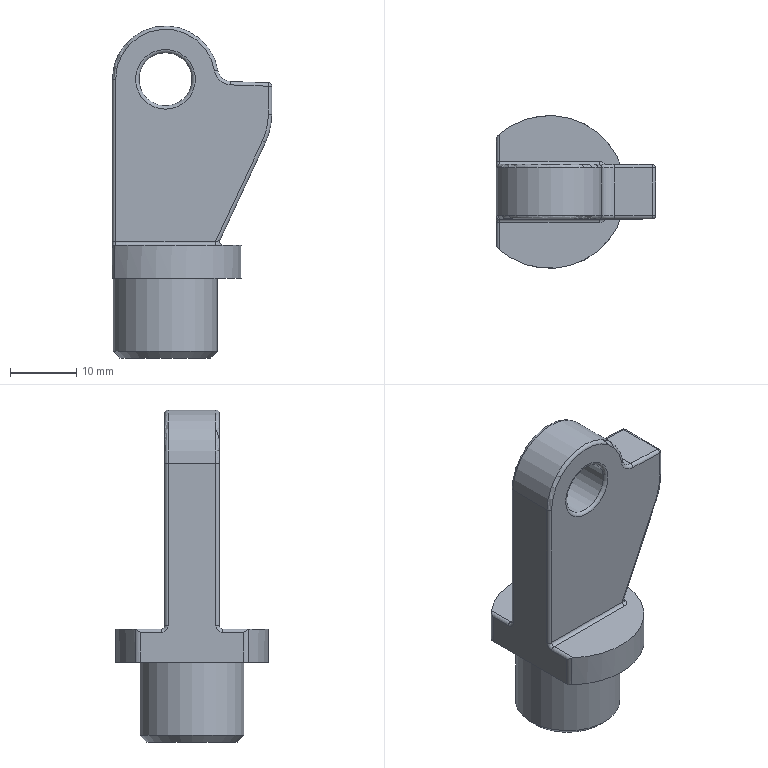Part | NX | features solid 2 | 1 solid | 46 faces | box 24 x 23 x 50 mm | volume 8887 mm3 | cylinder 22 | torus 10 | plane 9 | spline 2 | sphere 2 | cone 1 | commonest cylinder face diameters 1 x14 2 x2 4 x1 8 x1 15.7 x1 16 x1
STEP:
#1=CARTESIAN_POINT('',(15.517,-3.6,49.867));
#2=VERTEX_POINT('',#1);
#3=CARTESIAN_POINT('',(15.517,3.6,49.867));
#4=VERTEX_POINT('',#3);
#5=CARTESIAN_POINT('',(15.517,-7.201,49.867));
#6=DIRECTION('',(0.,1.,0.));
#7=VECTOR('',#6,1000.);
#8=LINE('',#5,#7);
#9=EDGE_CURVE('',#2,#4,#8,.T.);
#10=ORIENTED_EDGE('',*,*,#9,.T.);
#11=CARTESIAN_POINT('',(9.797,3.6,50.067));
#12=VERTEX_POINT('',#11);
#13=CARTESIAN_POINT('',(0.,3.6,50.409));
#14=DIRECTION('',(0.9994,0.,-0.0349));
#15=VECTOR('',#14,1000.);
#16=LINE('',#13,#15);
#17=EDGE_CURVE('',#4,#12,#16,.F.);
#18=ORIENTED_EDGE('',*,*,#17,.T.);
#19=CARTESIAN_POINT('',(9.797,-3.6,50.067));
#20=VERTEX_POINT('',#19);
#21=CARTESIAN_POINT('',(9.797,-4.1,50.067));
#22=DIRECTION('',(0.,-1.,0.));
#23=VECTOR('',#22,1000.);
#24=LINE('',#21,#23);
#25=EDGE_CURVE('',#12,#20,#24,.T.);
#26=ORIENTED_EDGE('',*,*,#25,.T.);
#27=CARTESIAN_POINT('',(0.,-3.6,50.409));
#28=DIRECTION('',(0.9994,0.,-0.0349));
#29=VECTOR('',#28,1000.);
#30=LINE('',#27,#29);
#31=EDGE_CURVE('',#20,#2,#30,.T.);
#32=ORIENTED_EDGE('',*,*,#31,.T.);
#33=EDGE_LOOP('',(#10,#18,#26,#32));
#34=FACE_BOUND('',#33,.T.);
#35=CARTESIAN_POINT('',(0.,-7.201,50.409));
#36=DIRECTION('',(-0.0349,0.,-0.9994));
#37=DIRECTION('',(0.,1.,0.));
#38=AXIS2_PLACEMENT_3D('',#35,#36,#37);
#39=PLANE('',#38);
#40=ADVANCED_FACE('',(#34),#39,.F.);
#41=CARTESIAN_POINT('',(0.,3.6,54.409));
#42=VERTEX_POINT('',#41);
#43=CARTESIAN_POINT('',(0.,3.6,50.409));
#44=DIRECTION('',(0.,1.,0.));
#45=DIRECTION('',(0.,0.,1.));
#46=AXIS2_PLACEMENT_3D('',#43,#44,#45);
#47=CIRCLE('',#46,4.);
#48=EDGE_CURVE('',#42,#42,#47,.T.);
#49=ORIENTED_EDGE('',*,*,#48,.T.);
#50=EDGE_LOOP('',(#49));
#51=FACE_BOUND('',#50,.T.);
#52=CARTESIAN_POINT('',(0.,-3.6,46.409));
#53=VERTEX_POINT('',#52);
#54=CARTESIAN_POINT('',(0.,-3.6,50.409));
#55=DIRECTION('',(0.,-1.,0.));
#56=DIRECTION('',(0.,0.,-1.));
#57=AXIS2_PLACEMENT_3D('',#54,#55,#56);
#58=CIRCLE('',#57,4.);
#59=EDGE_CURVE('',#53,#53,#58,.T.);
#60=ORIENTED_EDGE('',*,*,#59,.T.);
#61=EDGE_LOOP('',(#60));
#62=FACE_BOUND('',#61,.T.);
#63=CARTESIAN_POINT('',(0.,-4.201,50.409));
#64=DIRECTION('',(0.,1.,0.));
#65=DIRECTION('',(1.,0.,0.007504));
#66=AXIS2_PLACEMENT_3D('',#63,#64,#65);
#67=CYLINDRICAL_SURFACE('',#66,4.);
#68=ADVANCED_FACE('',(#51,#62),#67,.F.);
#69=ORIENTED_EDGE('',*,*,#25,.F.);
#70=CARTESIAN_POINT('',(7.893,3.6,51.74));
#71=VERTEX_POINT('',#70);
#72=CARTESIAN_POINT('',(9.867,3.6,52.065));
#73=DIRECTION('',(0.,1.,0.));
#74=DIRECTION('',(0.,0.,1.));
#75=AXIS2_PLACEMENT_3D('',#72,#73,#74);
#76=CIRCLE('',#75,2.);
#77=EDGE_CURVE('',#12,#71,#76,.T.);
#78=ORIENTED_EDGE('',*,*,#77,.T.);
#79=CARTESIAN_POINT('',(7.893,-3.6,51.74));
#80=VERTEX_POINT('',#79);
#81=CARTESIAN_POINT('',(7.893,0.,51.74));
#82=DIRECTION('',(0.,-1.,0.));
#83=VECTOR('',#82,1000.);
#84=LINE('',#81,#83);
#85=EDGE_CURVE('',#80,#71,#84,.F.);
#86=ORIENTED_EDGE('',*,*,#85,.F.);
#87=CARTESIAN_POINT('',(9.867,-3.6,52.065));
#88=DIRECTION('',(0.,-1.,0.));
#89=DIRECTION('',(0.,0.,-1.));
#90=AXIS2_PLACEMENT_3D('',#87,#88,#89);
#91=CIRCLE('',#90,2.);
#92=EDGE_CURVE('',#80,#20,#91,.T.);
#93=ORIENTED_EDGE('',*,*,#92,.T.);
#94=EDGE_LOOP('',(#69,#78,#86,#93));
#95=FACE_BOUND('',#94,.T.);
#96=CARTESIAN_POINT('',(9.867,0.,52.065));
#97=DIRECTION('',(0.,-1.,0.));
#98=DIRECTION('',(0.,0.,-1.));
#99=AXIS2_PLACEMENT_3D('',#96,#97,#98);
#100=CYLINDRICAL_SURFACE('',#99,2.);
#101=ADVANCED_FACE('',(#95),#100,.F.);
#102=CARTESIAN_POINT('',(0.,4.1,54.909));
#103=VERTEX_POINT('',#102);
#104=CARTESIAN_POINT('',(0.,4.1,50.409));
#105=DIRECTION('',(0.,1.,0.));
#106=DIRECTION('',(0.,0.,1.));
#107=AXIS2_PLACEMENT_3D('',#104,#105,#106);
#108=CIRCLE('',#107,4.5);
#109=EDGE_CURVE('',#103,#103,#108,.F.);
#110=ORIENTED_EDGE('',*,*,#109,.F.);
#111=EDGE_LOOP('',(#110));
#112=FACE_BOUND('',#111,.T.);
#113=ORIENTED_EDGE('',*,*,#48,.F.);
#114=EDGE_LOOP('',(#113));
#115=FACE_BOUND('',#114,.T.);
#116=CARTESIAN_POINT('',(0.,3.6,50.409));
#117=DIRECTION('',(0.,1.,0.));
#118=DIRECTION('',(0.,0.,1.));
#119=AXIS2_PLACEMENT_3D('',#116,#117,#118);
#120=TOROIDAL_SURFACE('',#119,4.5,0.5);
#121=ADVANCED_FACE('',(#112,#115),#120,.T.);
#122=CARTESIAN_POINT('',(16.,-3.6,45.155));
#123=VERTEX_POINT('',#122);
#124=CARTESIAN_POINT('',(16.,3.6,45.155));
#125=VERTEX_POINT('',#124);
#126=CARTESIAN_POINT('',(16.,0.,45.155));
#127=DIRECTION('',(0.,1.,0.));
#128=VECTOR('',#127,1000.);
#129=LINE('',#126,#128);
#130=EDGE_CURVE('',#123,#125,#129,.T.);
#131=ORIENTED_EDGE('',*,*,#130,.T.);
#132=CARTESIAN_POINT('',(16.,3.6,49.367));
#133=VERTEX_POINT('',#132);
#134=CARTESIAN_POINT('',(16.,3.6,42.909));
#135=DIRECTION('',(0.,0.,-1.));
#136=VECTOR('',#135,1000.);
#137=LINE('',#134,#136);
#138=EDGE_CURVE('',#125,#133,#137,.F.);
#139=ORIENTED_EDGE('',*,*,#138,.T.);
#140=CARTESIAN_POINT('',(16.,-3.6,49.367));
#141=VERTEX_POINT('',#140);
#142=CARTESIAN_POINT('',(16.,0.,49.367));
#143=DIRECTION('',(0.,-1.,0.));
#144=VECTOR('',#143,1000.);
#145=LINE('',#142,#144);
#146=EDGE_CURVE('',#133,#141,#145,.T.);
#147=ORIENTED_EDGE('',*,*,#146,.T.);
#148=CARTESIAN_POINT('',(16.,-3.6,42.909));
#149=DIRECTION('',(0.,0.,1.));
#150=VECTOR('',#149,1000.);
#151=LINE('',#148,#150);
#152=EDGE_CURVE('',#141,#123,#151,.F.);
#153=ORIENTED_EDGE('',*,*,#152,.T.);
#154=EDGE_LOOP('',(#131,#139,#147,#153));
#155=FACE_BOUND('',#154,.T.);
#156=CARTESIAN_POINT('',(16.,0.,42.909));
#157=DIRECTION('',(1.,0.,0.));
#158=DIRECTION('',(0.,0.,-1.));
#159=AXIS2_PLACEMENT_3D('',#156,#157,#158);
#160=PLANE('',#159);
#161=ADVANCED_FACE('',(#155),#160,.T.);
#162=ORIENTED_EDGE('',*,*,#59,.F.);
#163=EDGE_LOOP('',(#162));
#164=FACE_BOUND('',#163,.T.);
#165=CARTESIAN_POINT('',(0.,-4.1,45.909));
#166=VERTEX_POINT('',#165);
#167=CARTESIAN_POINT('',(0.,-4.1,50.409));
#168=DIRECTION('',(0.,-1.,0.));
#169=DIRECTION('',(0.,0.,-1.));
#170=AXIS2_PLACEMENT_3D('',#167,#168,#169);
#171=CIRCLE('',#170,4.5);
#172=EDGE_CURVE('',#166,#166,#171,.F.);
#173=ORIENTED_EDGE('',*,*,#172,.F.);
#174=EDGE_LOOP('',(#173));
#175=FACE_BOUND('',#174,.T.);
#176=CARTESIAN_POINT('',(0.,-3.6,50.409));
#177=DIRECTION('',(0.,-1.,0.));
#178=DIRECTION('',(0.,0.,-1.));
#179=AXIS2_PLACEMENT_3D('',#176,#177,#178);
#180=TOROIDAL_SURFACE('',#179,4.5,0.5);
#181=ADVANCED_FACE('',(#164,#175),#180,.T.);
#182=ORIENTED_EDGE('',*,*,#85,.T.);
#183=CARTESIAN_POINT('',(-8.,3.6,50.438));
#184=VERTEX_POINT('',#183);
#185=CARTESIAN_POINT('',(0.,3.6,50.438));
#186=DIRECTION('',(0.,1.,0.));
#187=DIRECTION('',(0.,0.,1.));
#188=AXIS2_PLACEMENT_3D('',#185,#186,#187);
#189=CIRCLE('',#188,8.);
#190=EDGE_CURVE('',#71,#184,#189,.F.);
#191=ORIENTED_EDGE('',*,*,#190,.T.);
#192=CARTESIAN_POINT('',(-8.,-3.6,50.438));
#193=VERTEX_POINT('',#192);
#194=CARTESIAN_POINT('',(-8.,4.1,50.438));
#195=DIRECTION('',(0.,1.,0.));
#196=VECTOR('',#195,1000.);
#197=LINE('',#194,#196);
#198=EDGE_CURVE('',#193,#184,#197,.T.);
#199=ORIENTED_EDGE('',*,*,#198,.F.);
#200=CARTESIAN_POINT('',(0.,-3.6,50.438));
#201=DIRECTION('',(0.,-1.,0.));
#202=DIRECTION('',(0.,0.,-1.));
#203=AXIS2_PLACEMENT_3D('',#200,#201,#202);
#204=CIRCLE('',#203,8.);
#205=EDGE_CURVE('',#193,#80,#204,.F.);
#206=ORIENTED_EDGE('',*,*,#205,.T.);
#207=EDGE_LOOP('',(#182,#191,#199,#206));
#208=FACE_BOUND('',#207,.T.);
#209=CARTESIAN_POINT('',(0.,0.,50.438));
#210=DIRECTION('',(0.,-1.,0.));
#211=DIRECTION('',(0.,0.,-1.));
#212=AXIS2_PLACEMENT_3D('',#209,#210,#211);
#213=CYLINDRICAL_SURFACE('',#212,8.);
#214=ADVANCED_FACE('',(#208),#213,.T.);
#215=CARTESIAN_POINT('',(8.171,-3.6,26.149));
#216=VERTEX_POINT('',#215);
#217=CARTESIAN_POINT('',(8.171,3.6,26.149));
#218=VERTEX_POINT('',#217);
#219=CARTESIAN_POINT('',(8.171,4.1,26.149));
#220=DIRECTION('',(0.,-1.,0.));
#221=VECTOR('',#220,1000.);
#222=LINE('',#219,#221);
#223=EDGE_CURVE('',#216,#218,#222,.F.);
#224=ORIENTED_EDGE('',*,*,#223,.T.);
#225=CARTESIAN_POINT('',(15.063,3.6,40.929));
#226=VERTEX_POINT('',#225);
#227=CARTESIAN_POINT('',(16.,3.6,42.938));
#228=DIRECTION('',(-0.4226,0.,-0.9063));
#229=VECTOR('',#228,1000.);
#230=LINE('',#227,#229);
#231=EDGE_CURVE('',#218,#226,#230,.F.);
#232=ORIENTED_EDGE('',*,*,#231,.T.);
#233=CARTESIAN_POINT('',(15.063,-3.6,40.929));
#234=VERTEX_POINT('',#233);
#235=CARTESIAN_POINT('',(15.063,0.,40.929));
#236=DIRECTION('',(0.,1.,0.));
#237=VECTOR('',#236,1000.);
#238=LINE('',#235,#237);
#239=EDGE_CURVE('',#226,#234,#238,.F.);
#240=ORIENTED_EDGE('',*,*,#239,.T.);
#241=CARTESIAN_POINT('',(16.,-3.6,42.938));
#242=DIRECTION('',(0.4226,0.,0.9063));
#243=VECTOR('',#242,1000.);
#244=LINE('',#241,#243);
#245=EDGE_CURVE('',#234,#216,#244,.F.);
#246=ORIENTED_EDGE('',*,*,#245,.T.);
#247=EDGE_LOOP('',(#224,#232,#240,#246));
#248=FACE_BOUND('',#247,.T.);
#249=CARTESIAN_POINT('',(16.,0.,42.938));
#250=DIRECTION('',(0.9063,0.,-0.4226));
#251=DIRECTION('',(-0.4226,0.,-0.9063));
#252=AXIS2_PLACEMENT_3D('',#249,#250,#251);
#253=PLANE('',#252);
#254=ADVANCED_FACE('',(#248),#253,.T.);
#255=CARTESIAN_POINT('',(-8.,7.826,24.938));
#256=VERTEX_POINT('',#255);
#257=CARTESIAN_POINT('',(-8.,4.6,24.938));
#258=VERTEX_POINT('',#257);
#259=CARTESIAN_POINT('',(-8.,8.261,24.938));
#260=DIRECTION('',(0.,-1.,0.));
#261=VECTOR('',#260,1000.);
#262=LINE('',#259,#261);
#263=EDGE_CURVE('',#256,#258,#262,.T.);
#264=ORIENTED_EDGE('',*,*,#263,.F.);
#265=CARTESIAN_POINT('',(-8.,7.826,20.438));
#266=VERTEX_POINT('',#265);
#267=CARTESIAN_POINT('',(-8.,7.826,36.483));
#268=DIRECTION('',(0.,0.,1.));
#269=VECTOR('',#268,1000.);
#270=LINE('',#267,#269);
#271=EDGE_CURVE('',#256,#266,#270,.F.);
#272=ORIENTED_EDGE('',*,*,#271,.T.);
#273=CARTESIAN_POINT('',(-8.,-7.826,20.438));
#274=VERTEX_POINT('',#273);
#275=CARTESIAN_POINT('',(-8.,0.,20.438));
#276=DIRECTION('',(0.,1.,0.));
#277=VECTOR('',#276,1000.);
#278=LINE('',#275,#277);
#279=EDGE_CURVE('',#274,#266,#278,.T.);
#280=ORIENTED_EDGE('',*,*,#279,.F.);
#281=CARTESIAN_POINT('',(-8.,-7.826,24.938));
#282=VERTEX_POINT('',#281);
#283=CARTESIAN_POINT('',(-8.,-7.826,36.483));
#284=DIRECTION('',(0.,0.,1.));
#285=VECTOR('',#284,1000.);
#286=LINE('',#283,#285);
#287=EDGE_CURVE('',#274,#282,#286,.T.);
#288=ORIENTED_EDGE('',*,*,#287,.T.);
#289=CARTESIAN_POINT('',(-8.,-4.6,24.938));
#290=VERTEX_POINT('',#289);
#291=CARTESIAN_POINT('',(-8.,-4.1,24.938));
#292=DIRECTION('',(0.,-1.,0.));
#293=VECTOR('',#292,1000.);
#294=LINE('',#291,#293);
#295=EDGE_CURVE('',#282,#290,#294,.F.);
#296=ORIENTED_EDGE('',*,*,#295,.T.);
#297=CARTESIAN_POINT('',(-8.,-3.6,25.938));
#298=VERTEX_POINT('',#297);
#299=CARTESIAN_POINT('',(-8.,-4.6,25.938));
#300=DIRECTION('',(1.,0.,0.));
#301=DIRECTION('',(0.,0.,-1.));
#302=AXIS2_PLACEMENT_3D('',#299,#300,#301);
#303=CIRCLE('',#302,1.);
#304=EDGE_CURVE('',#298,#290,#303,.F.);
#305=ORIENTED_EDGE('',*,*,#304,.F.);
#306=CARTESIAN_POINT('',(-8.,-3.6,50.438));
#307=DIRECTION('',(0.,0.,1.));
#308=VECTOR('',#307,1000.);
#309=LINE('',#306,#308);
#310=EDGE_CURVE('',#193,#298,#309,.F.);
#311=ORIENTED_EDGE('',*,*,#310,.F.);
#312=ORIENTED_EDGE('',*,*,#198,.T.);
#313=CARTESIAN_POINT('',(-8.,3.6,25.938));
#314=VERTEX_POINT('',#313);
#315=CARTESIAN_POINT('',(-8.,3.6,25.438));
#316=DIRECTION('',(0.,0.,1.));
#317=VECTOR('',#316,1000.);
#318=LINE('',#315,#317);
#319=EDGE_CURVE('',#184,#314,#318,.F.);
#320=ORIENTED_EDGE('',*,*,#319,.T.);
#321=CARTESIAN_POINT('',(-8.,4.6,25.938));
#322=DIRECTION('',(1.,0.,0.));
#323=DIRECTION('',(0.,0.,-1.));
#324=AXIS2_PLACEMENT_3D('',#321,#322,#323);
#325=CIRCLE('',#324,1.);
#326=EDGE_CURVE('',#258,#314,#325,.F.);
#327=ORIENTED_EDGE('',*,*,#326,.F.);
#328=EDGE_LOOP('',(#264,#272,#280,#288,#296,#305,#311,#312,#320,#327));
#329=FACE_BOUND('',#328,.T.);
#330=CARTESIAN_POINT('',(-8.,0.,36.483));
#331=DIRECTION('',(1.,0.,0.));
#332=DIRECTION('',(0.,0.,-1.));
#333=AXIS2_PLACEMENT_3D('',#330,#331,#332);
#334=PLANE('',#333);
#335=ADVANCED_FACE('',(#329),#334,.F.);
#336=CARTESIAN_POINT('',(15.5,-4.1,49.367));
#337=VERTEX_POINT('',#336);
#338=CARTESIAN_POINT('',(9.779,-4.1,49.567));
#339=VERTEX_POINT('',#338);
#340=CARTESIAN_POINT('',(0.7194,-4.1,49.883));
#341=DIRECTION('',(-0.9994,0.,0.0349));
#342=VECTOR('',#341,1000.);
#343=LINE('',#340,#342);
#344=EDGE_CURVE('',#337,#339,#343,.T.);
#345=ORIENTED_EDGE('',*,*,#344,.T.);
#346=CARTESIAN_POINT('',(7.4,-4.1,51.659));
#347=VERTEX_POINT('',#346);
#348=CARTESIAN_POINT('',(9.867,-4.1,52.065));
#349=DIRECTION('',(0.,-1.,0.));
#350=DIRECTION('',(0.,0.,-1.));
#351=AXIS2_PLACEMENT_3D('',#348,#349,#350);
#352=CIRCLE('',#351,2.5);
#353=EDGE_CURVE('',#339,#347,#352,.F.);
#354=ORIENTED_EDGE('',*,*,#353,.T.);
#355=CARTESIAN_POINT('',(-7.5,-4.1,50.438));
#356=VERTEX_POINT('',#355);
#357=CARTESIAN_POINT('',(0.,-4.1,50.438));
#358=DIRECTION('',(0.,-1.,0.));
#359=DIRECTION('',(0.,0.,-1.));
#360=AXIS2_PLACEMENT_3D('',#357,#358,#359);
#361=CIRCLE('',#360,7.5);
#362=EDGE_CURVE('',#347,#356,#361,.T.);
#363=ORIENTED_EDGE('',*,*,#362,.T.);
#364=CARTESIAN_POINT('',(-7.5,-4.1,25.938));
#365=VERTEX_POINT('',#364);
#366=CARTESIAN_POINT('',(-7.5,-4.1,25.438));
#367=DIRECTION('',(0.,0.,1.));
#368=VECTOR('',#367,1000.);
#369=LINE('',#366,#368);
#370=EDGE_CURVE('',#356,#365,#369,.F.);
#371=ORIENTED_EDGE('',*,*,#370,.T.);
#372=CARTESIAN_POINT('',(7.521,-4.1,25.938));
#373=VERTEX_POINT('',#372);
#374=CARTESIAN_POINT('',(7.84,-4.1,25.938));
#375=DIRECTION('',(1.,0.,0.));
#376=VECTOR('',#375,1000.);
#377=LINE('',#374,#376);
#378=EDGE_CURVE('',#365,#373,#377,.T.);
#379=ORIENTED_EDGE('',*,*,#378,.T.);
#380=CARTESIAN_POINT('',(14.61,-4.1,41.14));
#381=VERTEX_POINT('',#380);
#382=CARTESIAN_POINT('',(7.459,-4.1,25.805));
#383=DIRECTION('',(0.4226,0.,0.9063));
#384=VECTOR('',#383,1000.);
#385=LINE('',#382,#384);
#386=EDGE_CURVE('',#373,#381,#385,.T.);
#387=ORIENTED_EDGE('',*,*,#386,.T.);
#388=CARTESIAN_POINT('',(15.5,-4.1,45.155));
#389=VERTEX_POINT('',#388);
#390=CARTESIAN_POINT('',(6.,-4.1,45.155));
#391=DIRECTION('',(0.,-1.,0.));
#392=DIRECTION('',(0.,0.,-1.));
#393=AXIS2_PLACEMENT_3D('',#390,#391,#392);
#394=CIRCLE('',#393,9.5);
#395=EDGE_CURVE('',#381,#389,#394,.T.);
#396=ORIENTED_EDGE('',*,*,#395,.T.);
#397=CARTESIAN_POINT('',(15.5,-4.1,29.284));
#398=DIRECTION('',(0.,0.,1.));
#399=VECTOR('',#398,1000.);
#400=LINE('',#397,#399);
#401=EDGE_CURVE('',#389,#337,#400,.T.);
#402=ORIENTED_EDGE('',*,*,#401,.T.);
#403=EDGE_LOOP('',(#345,#354,#363,#371,#379,#387,#396,#402));
#404=FACE_BOUND('',#403,.T.);
#405=ORIENTED_EDGE('',*,*,#172,.T.);
#406=EDGE_LOOP('',(#405));
#407=FACE_BOUND('',#406,.T.);
#408=CARTESIAN_POINT('',(0.,-4.1,29.284));
#409=DIRECTION('',(0.,-1.,0.));
#410=DIRECTION('',(0.,0.,-1.));
#411=AXIS2_PLACEMENT_3D('',#408,#409,#410);
#412=PLANE('',#411);
#413=ADVANCED_FACE('',(#404,#407),#412,.T.);
#414=CARTESIAN_POINT('',(9.779,4.1,49.567));
#415=VERTEX_POINT('',#414);
#416=CARTESIAN_POINT('',(15.5,4.1,49.367));
#417=VERTEX_POINT('',#416);
#418=CARTESIAN_POINT('',(0.7194,4.1,49.883));
#419=DIRECTION('',(-0.9994,0.,0.0349));
#420=VECTOR('',#419,1000.);
#421=LINE('',#418,#420);
#422=EDGE_CURVE('',#415,#417,#421,.F.);
#423=ORIENTED_EDGE('',*,*,#422,.T.);
#424=CARTESIAN_POINT('',(15.5,4.1,45.155));
#425=VERTEX_POINT('',#424);
#426=CARTESIAN_POINT('',(15.5,4.1,29.284));
#427=DIRECTION('',(0.,0.,-1.));
#428=VECTOR('',#427,1000.);
#429=LINE('',#426,#428);
#430=EDGE_CURVE('',#417,#425,#429,.T.);
#431=ORIENTED_EDGE('',*,*,#430,.T.);
#432=CARTESIAN_POINT('',(14.61,4.1,41.14));
#433=VERTEX_POINT('',#432);
#434=CARTESIAN_POINT('',(6.,4.1,45.155));
#435=DIRECTION('',(0.,1.,0.));
#436=DIRECTION('',(0.,0.,1.));
#437=AXIS2_PLACEMENT_3D('',#434,#435,#436);
#438=CIRCLE('',#437,9.5);
#439=EDGE_CURVE('',#425,#433,#438,.T.);
#440=ORIENTED_EDGE('',*,*,#439,.T.);
#441=CARTESIAN_POINT('',(7.521,4.1,25.938));
#442=VERTEX_POINT('',#441);
#443=CARTESIAN_POINT('',(7.459,4.1,25.805));
#444=DIRECTION('',(-0.4226,0.,-0.9063));
#445=VECTOR('',#444,1000.);
#446=LINE('',#443,#445);
#447=EDGE_CURVE('',#433,#442,#446,.T.);
#448=ORIENTED_EDGE('',*,*,#447,.T.);
#449=CARTESIAN_POINT('',(-7.5,4.1,25.938));
#450=VERTEX_POINT('',#449);
#451=CARTESIAN_POINT('',(-8.,4.1,25.938));
#452=DIRECTION('',(1.,0.,0.));
#453=VECTOR('',#452,1000.);
#454=LINE('',#451,#453);
#455=EDGE_CURVE('',#442,#450,#454,.F.);
#456=ORIENTED_EDGE('',*,*,#455,.T.);
#457=CARTESIAN_POINT('',(-7.5,4.1,50.438));
#458=VERTEX_POINT('',#457);
#459=CARTESIAN_POINT('',(-7.5,4.1,50.438));
#460=DIRECTION('',(0.,0.,1.));
#461=VECTOR('',#460,1000.);
#462=LINE('',#459,#461);
#463=EDGE_CURVE('',#450,#458,#462,.T.);
#464=ORIENTED_EDGE('',*,*,#463,.T.);
#465=CARTESIAN_POINT('',(7.4,4.1,51.659));
#466=VERTEX_POINT('',#465);
#467=CARTESIAN_POINT('',(0.,4.1,50.438));
#468=DIRECTION('',(0.,1.,0.));
#469=DIRECTION('',(0.,0.,1.));
#470=AXIS2_PLACEMENT_3D('',#467,#468,#469);
#471=CIRCLE('',#470,7.5);
#472=EDGE_CURVE('',#458,#466,#471,.T.);
#473=ORIENTED_EDGE('',*,*,#472,.T.);
#474=CARTESIAN_POINT('',(9.867,4.1,52.065));
#475=DIRECTION('',(0.,1.,0.));
#476=DIRECTION('',(0.,0.,1.));
#477=AXIS2_PLACEMENT_3D('',#474,#475,#476);
#478=CIRCLE('',#477,2.5);
#479=EDGE_CURVE('',#466,#415,#478,.F.);
#480=ORIENTED_EDGE('',*,*,#479,.T.);
#481=EDGE_LOOP('',(#423,#431,#440,#448,#456,#464,#473,#480));
#482=FACE_BOUND('',#481,.T.);
#483=ORIENTED_EDGE('',*,*,#109,.T.);
#484=EDGE_LOOP('',(#483));
#485=FACE_BOUND('',#484,.T.);
#486=CARTESIAN_POINT('',(0.,4.1,29.284));
#487=DIRECTION('',(0.,1.,0.));
#488=DIRECTION('',(0.,0.,-1.));
#489=AXIS2_PLACEMENT_3D('',#486,#487,#488);
#490=PLANE('',#489);
#491=ADVANCED_FACE('',(#482,#485),#490,.T.);
#492=ORIENTED_EDGE('',*,*,#239,.F.);
#493=CARTESIAN_POINT('',(6.,3.6,45.155));
#494=DIRECTION('',(0.,1.,0.));
#495=DIRECTION('',(0.,0.,1.));
#496=AXIS2_PLACEMENT_3D('',#493,#494,#495);
#497=CIRCLE('',#496,10.);
#498=EDGE_CURVE('',#226,#125,#497,.F.);
#499=ORIENTED_EDGE('',*,*,#498,.T.);
#500=ORIENTED_EDGE('',*,*,#130,.F.);
#501=CARTESIAN_POINT('',(6.,-3.6,45.155));
#502=DIRECTION('',(0.,-1.,0.));
#503=DIRECTION('',(0.,0.,-1.));
#504=AXIS2_PLACEMENT_3D('',#501,#502,#503);
#505=CIRCLE('',#504,10.);
#506=EDGE_CURVE('',#123,#234,#505,.F.);
#507=ORIENTED_EDGE('',*,*,#506,.T.);
#508=EDGE_LOOP('',(#492,#499,#500,#507));
#509=FACE_BOUND('',#508,.T.);
#510=CARTESIAN_POINT('',(6.,0.,45.155));
#511=DIRECTION('',(0.,1.,0.));
#512=DIRECTION('',(0.,0.,1.));
#513=AXIS2_PLACEMENT_3D('',#510,#511,#512);
#514=CYLINDRICAL_SURFACE('',#513,10.);
#515=ADVANCED_FACE('',(#509),#514,.T.);
#516=CARTESIAN_POINT('',(-7.5,-8.718,25.438));
#517=VERTEX_POINT('',#516);
#518=CARTESIAN_POINT('',(-7.5,8.718,25.438));
#519=VERTEX_POINT('',#518);
#520=CARTESIAN_POINT('',(0.,0.,25.438));
#521=DIRECTION('',(0.,0.,1.));
#522=DIRECTION('',(1.,0.,0.));
#523=AXIS2_PLACEMENT_3D('',#520,#521,#522);
#524=CIRCLE('',#523,11.5);
#525=EDGE_CURVE('',#517,#519,#524,.T.);
#526=ORIENTED_EDGE('',*,*,#525,.T.);
#527=CARTESIAN_POINT('',(-7.5,4.6,25.438));
#528=VERTEX_POINT('',#527);
#529=CARTESIAN_POINT('',(-7.5,4.1,25.438));
#530=DIRECTION('',(0.,-1.,0.));
#531=VECTOR('',#530,1000.);
#532=LINE('',#529,#531);
#533=EDGE_CURVE('',#519,#528,#532,.T.);
#534=ORIENTED_EDGE('',*,*,#533,.T.);
#535=CARTESIAN_POINT('',(7.521,4.6,25.438));
#536=VERTEX_POINT('',#535);
#537=CARTESIAN_POINT('',(7.84,4.6,25.438));
#538=DIRECTION('',(1.,0.,0.));
#539=VECTOR('',#538,1000.);
#540=LINE('',#537,#539);
#541=EDGE_CURVE('',#528,#536,#540,.T.);
#542=ORIENTED_EDGE('',*,*,#541,.T.);
#543=CARTESIAN_POINT('',(8.624,3.6,25.438));
#544=VERTEX_POINT('',#543);
#545=CARTESIAN_POINT('',(7.521,3.6,25.438));
#546=DIRECTION('',(0.,0.,1.));
#547=DIRECTION('',(-1.,0.,0.));
#548=AXIS2_PLACEMENT_3D('',#545,#546,#547);
#549=ELLIPSE('',#548,1.103,1.);
#550=EDGE_CURVE('',#544,#536,#549,.T.);
#551=ORIENTED_EDGE('',*,*,#550,.F.);
#552=CARTESIAN_POINT('',(8.624,-3.6,25.438));
#553=VERTEX_POINT('',#552);
#554=CARTESIAN_POINT('',(8.624,-4.1,25.438));
#555=DIRECTION('',(0.,-1.,0.));
#556=VECTOR('',#555,1000.);
#557=LINE('',#554,#556);
#558=EDGE_CURVE('',#553,#544,#557,.F.);
#559=ORIENTED_EDGE('',*,*,#558,.F.);
#560=CARTESIAN_POINT('',(7.521,-4.6,25.438));
#561=VERTEX_POINT('',#560);
#562=CARTESIAN_POINT('',(7.521,-3.6,25.438));
#563=DIRECTION('',(0.,0.,1.));
#564=DIRECTION('',(1.,0.,0.));
#565=AXIS2_PLACEMENT_3D('',#562,#563,#564);
#566=ELLIPSE('',#565,1.103,1.);
#567=EDGE_CURVE('',#561,#553,#566,.T.);
#568=ORIENTED_EDGE('',*,*,#567,.F.);
#569=CARTESIAN_POINT('',(-7.5,-4.6,25.438));
#570=VERTEX_POINT('',#569);
#571=CARTESIAN_POINT('',(-8.,-4.6,25.438));
#572=DIRECTION('',(1.,0.,0.));
#573=VECTOR('',#572,1000.);
#574=LINE('',#571,#573);
#575=EDGE_CURVE('',#561,#570,#574,.F.);
#576=ORIENTED_EDGE('',*,*,#575,.T.);
#577=CARTESIAN_POINT('',(-7.5,-8.261,25.438));
#578=DIRECTION('',(0.,-1.,0.));
#579=VECTOR('',#578,1000.);
#580=LINE('',#577,#579);
#581=EDGE_CURVE('',#570,#517,#580,.T.);
#582=ORIENTED_EDGE('',*,*,#581,.T.);
#583=EDGE_LOOP('',(#526,#534,#542,#551,#559,#568,#576,#582));
#584=FACE_BOUND('',#583,.T.);
#585=CARTESIAN_POINT('',(0.,0.,25.438));
#586=DIRECTION('',(0.,0.,1.));
#587=DIRECTION('',(1.,0.,0.));
#588=AXIS2_PLACEMENT_3D('',#585,#586,#587);
#589=PLANE('',#588);
#590=ADVANCED_FACE('',(#584),#589,.T.);
#591=CARTESIAN_POINT('',(-7.667,-8.572,20.438));
#592=VERTEX_POINT('',#591);
#593=CARTESIAN_POINT('',(-7.667,8.572,20.438));
#594=VERTEX_POINT('',#593);
#595=CARTESIAN_POINT('',(0.,0.,20.438));
#596=DIRECTION('',(0.,0.,1.));
#597=DIRECTION('',(1.,0.,0.));
#598=AXIS2_PLACEMENT_3D('',#595,#596,#597);
#599=CIRCLE('',#598,11.5);
#600=EDGE_CURVE('',#592,#594,#599,.T.);
#601=ORIENTED_EDGE('',*,*,#600,.T.);
#602=CARTESIAN_POINT('',(-7.667,8.572,25.409));
#603=VERTEX_POINT('',#602);
#604=CARTESIAN_POINT('',(-7.667,8.572,40.162));
#605=DIRECTION('',(0.,0.,1.));
#606=VECTOR('',#605,1000.);
#607=LINE('',#604,#606);
#608=EDGE_CURVE('',#594,#603,#607,.T.);
#609=ORIENTED_EDGE('',*,*,#608,.T.);
#610=CARTESIAN_POINT('',(-7.667,8.572,25.409));
#611=CARTESIAN_POINT('',(-7.613,8.62,25.428));
#612=CARTESIAN_POINT('',(-7.557,8.669,25.438));
#613=CARTESIAN_POINT('',(-7.5,8.718,25.438));
#614=B_SPLINE_CURVE_WITH_KNOTS('',3,(#610,#611,#612,#613),.UNSPECIFIED.,.F.,.F.,(4,4),(0.000701,0.0009241),.UNSPECIFIED.);
#615=EDGE_CURVE('',#603,#519,#614,.T.);
#616=ORIENTED_EDGE('',*,*,#615,.T.);
#617=ORIENTED_EDGE('',*,*,#525,.F.);
#618=CARTESIAN_POINT('',(-7.667,-8.572,25.409));
#619=VERTEX_POINT('',#618);
#620=CARTESIAN_POINT('',(-7.5,-8.718,25.438));
#621=CARTESIAN_POINT('',(-7.557,-8.669,25.438));
#622=CARTESIAN_POINT('',(-7.613,-8.62,25.428));
#623=CARTESIAN_POINT('',(-7.667,-8.572,25.409));
#624=B_SPLINE_CURVE_WITH_KNOTS('',3,(#620,#621,#622,#623),.UNSPECIFIED.,.F.,.F.,(4,4),(0.,0.0002235),.UNSPECIFIED.);
#625=EDGE_CURVE('',#517,#619,#624,.T.);
#626=ORIENTED_EDGE('',*,*,#625,.T.);
#627=CARTESIAN_POINT('',(-7.667,-8.572,40.162));
#628=DIRECTION('',(0.,0.,1.));
#629=VECTOR('',#628,1000.);
#630=LINE('',#627,#629);
#631=EDGE_CURVE('',#619,#592,#630,.F.);
#632=ORIENTED_EDGE('',*,*,#631,.T.);
#633=EDGE_LOOP('',(#601,#609,#616,#617,#626,#632));
#634=FACE_BOUND('',#633,.T.);
#635=CARTESIAN_POINT('',(0.,0.,40.162));
#636=DIRECTION('',(0.,0.,1.));
#637=DIRECTION('',(0.,-1.,0.));
#638=AXIS2_PLACEMENT_3D('',#635,#636,#637);
#639=CYLINDRICAL_SURFACE('',#638,11.5);
#640=ADVANCED_FACE('',(#634),#639,.T.);
#641=CARTESIAN_POINT('',(6.85,0.,8.438));
#642=VERTEX_POINT('',#641);
#643=CARTESIAN_POINT('',(0.,0.,8.438));
#644=DIRECTION('',(0.,0.,1.));
#645=DIRECTION('',(1.,0.,0.));
#646=AXIS2_PLACEMENT_3D('',#643,#644,#645);
#647=CIRCLE('',#646,6.85);
#648=EDGE_CURVE('',#642,#642,#647,.F.);
#649=ORIENTED_EDGE('',*,*,#648,.T.);
#650=EDGE_LOOP('',(#649));
#651=FACE_BOUND('',#650,.T.);
#652=CARTESIAN_POINT('',(6.223,0.,8.438));
#653=DIRECTION('',(0.,0.,1.));
#654=DIRECTION('',(0.,-1.,0.));
#655=AXIS2_PLACEMENT_3D('',#652,#653,#654);
#656=PLANE('',#655);
#657=ADVANCED_FACE('',(#651),#656,.F.);
#658=ORIENTED_EDGE('',*,*,#279,.T.);
#659=CARTESIAN_POINT('',(-7.,7.826,20.438));
#660=DIRECTION('',(0.,0.,1.));
#661=DIRECTION('',(1.,0.,0.));
#662=AXIS2_PLACEMENT_3D('',#659,#660,#661);
#663=CIRCLE('',#662,1.);
#664=EDGE_CURVE('',#266,#594,#663,.F.);
#665=ORIENTED_EDGE('',*,*,#664,.T.);
#666=ORIENTED_EDGE('',*,*,#600,.F.);
#667=CARTESIAN_POINT('',(-7.,-7.826,20.438));
#668=DIRECTION('',(0.,0.,1.));
#669=DIRECTION('',(1.,0.,0.));
#670=AXIS2_PLACEMENT_3D('',#667,#668,#669);
#671=CIRCLE('',#670,1.);
#672=EDGE_CURVE('',#592,#274,#671,.F.);
#673=ORIENTED_EDGE('',*,*,#672,.T.);
#674=EDGE_LOOP('',(#658,#665,#666,#673));
#675=FACE_BOUND('',#674,.T.);
#676=CARTESIAN_POINT('',(7.85,0.,20.438));
#677=VERTEX_POINT('',#676);
#678=CARTESIAN_POINT('',(0.,0.,20.438));
#679=DIRECTION('',(0.,0.,1.));
#680=DIRECTION('',(1.,0.,0.));
#681=AXIS2_PLACEMENT_3D('',#678,#679,#680);
#682=CIRCLE('',#681,7.85);
#683=EDGE_CURVE('',#677,#677,#682,.F.);
#684=ORIENTED_EDGE('',*,*,#683,.F.);
#685=EDGE_LOOP('',(#684));
#686=FACE_BOUND('',#685,.T.);
#687=CARTESIAN_POINT('',(0.,0.,20.438));
#688=DIRECTION('',(0.,0.,1.));
#689=DIRECTION('',(1.,0.,0.));
#690=AXIS2_PLACEMENT_3D('',#687,#688,#689);
#691=PLANE('',#690);
#692=ADVANCED_FACE('',(#675,#686),#691,.F.);
#693=CARTESIAN_POINT('',(7.85,0.,9.438));
#694=VERTEX_POINT('',#693);
#695=CARTESIAN_POINT('',(0.,0.,9.438));
#696=DIRECTION('',(0.,0.,1.));
#697=DIRECTION('',(1.,0.,0.));
#698=AXIS2_PLACEMENT_3D('',#695,#696,#697);
#699=CIRCLE('',#698,7.85);
#700=EDGE_CURVE('',#694,#694,#699,.T.);
#701=ORIENTED_EDGE('',*,*,#700,.T.);
#702=EDGE_LOOP('',(#701));
#703=FACE_BOUND('',#702,.T.);
#704=ORIENTED_EDGE('',*,*,#683,.T.);
#705=EDGE_LOOP('',(#704));
#706=FACE_BOUND('',#705,.T.);
#707=CARTESIAN_POINT('',(0.,0.,40.162));
#708=DIRECTION('',(0.,0.,1.));
#709=DIRECTION('',(0.,-1.,0.));
#710=AXIS2_PLACEMENT_3D('',#707,#708,#709);
#711=CYLINDRICAL_SURFACE('',#710,7.85);
#712=ADVANCED_FACE('',(#703,#706),#711,.T.);
#713=ORIENTED_EDGE('',*,*,#700,.F.);
#714=EDGE_LOOP('',(#713));
#715=FACE_BOUND('',#714,.T.);
#716=ORIENTED_EDGE('',*,*,#648,.F.);
#717=EDGE_LOOP('',(#716));
#718=FACE_BOUND('',#717,.T.);
#719=CARTESIAN_POINT('',(0.,0.,8.438));
#720=DIRECTION('',(0.,0.,1.));
#721=DIRECTION('',(1.,0.,0.));
#722=AXIS2_PLACEMENT_3D('',#719,#720,#721);
#723=CONICAL_SURFACE('',#722,6.85,0.7854);
#724=ADVANCED_FACE('',(#715,#718),#723,.T.);
#725=ORIENTED_EDGE('',*,*,#295,.F.);
#726=CARTESIAN_POINT('',(-7.667,-8.572,25.409));
#727=CARTESIAN_POINT('',(-7.902,-8.361,25.326));
#728=CARTESIAN_POINT('',(-8.,-8.09,25.124));
#729=CARTESIAN_POINT('',(-8.,-7.826,24.938));
#730=B_SPLINE_CURVE_WITH_KNOTS('',3,(#726,#727,#728,#729),.UNSPECIFIED.,.F.,.F.,(4,4),(0.,0.0009677),.UNSPECIFIED.);
#731=EDGE_CURVE('',#282,#619,#730,.F.);
#732=ORIENTED_EDGE('',*,*,#731,.T.);
#733=ORIENTED_EDGE('',*,*,#625,.F.);
#734=ORIENTED_EDGE('',*,*,#581,.F.);
#735=CARTESIAN_POINT('',(-7.5,-4.6,24.938));
#736=DIRECTION('',(0.,1.,0.));
#737=DIRECTION('',(0.,0.,1.));
#738=AXIS2_PLACEMENT_3D('',#735,#736,#737);
#739=CIRCLE('',#738,0.5);
#740=EDGE_CURVE('',#290,#570,#739,.T.);
#741=ORIENTED_EDGE('',*,*,#740,.F.);
#742=EDGE_LOOP('',(#725,#732,#733,#734,#741));
#743=FACE_BOUND('',#742,.T.);
#744=CARTESIAN_POINT('',(-7.5,0.,24.938));
#745=DIRECTION('',(0.,1.,0.));
#746=DIRECTION('',(0.,0.,1.));
#747=AXIS2_PLACEMENT_3D('',#744,#745,#746);
#748=CYLINDRICAL_SURFACE('',#747,0.5);
#749=ADVANCED_FACE('',(#743),#748,.T.);
#750=CARTESIAN_POINT('',(-7.5,-3.6,50.438));
#751=DIRECTION('',(0.,0.,1.));
#752=DIRECTION('',(1.,0.,0.));
#753=AXIS2_PLACEMENT_3D('',#750,#751,#752);
#754=CIRCLE('',#753,0.5);
#755=EDGE_CURVE('',#356,#193,#754,.F.);
#756=ORIENTED_EDGE('',*,*,#755,.T.);
#757=ORIENTED_EDGE('',*,*,#310,.T.);
#758=CARTESIAN_POINT('',(-7.5,-3.6,25.938));
#759=DIRECTION('',(0.,0.,-1.));
#760=DIRECTION('',(-1.,0.,0.));
#761=AXIS2_PLACEMENT_3D('',#758,#759,#760);
#762=CIRCLE('',#761,0.5);
#763=EDGE_CURVE('',#365,#298,#762,.T.);
#764=ORIENTED_EDGE('',*,*,#763,.F.);
#765=ORIENTED_EDGE('',*,*,#370,.F.);
#766=EDGE_LOOP('',(#756,#757,#764,#765));
#767=FACE_BOUND('',#766,.T.);
#768=CARTESIAN_POINT('',(-7.5,-3.6,36.483));
#769=DIRECTION('',(0.,0.,-1.));
#770=DIRECTION('',(-1.,0.,0.));
#771=AXIS2_PLACEMENT_3D('',#768,#769,#770);
#772=CYLINDRICAL_SURFACE('',#771,0.5);
#773=ADVANCED_FACE('',(#767),#772,.T.);
#774=ORIENTED_EDGE('',*,*,#304,.T.);
#775=ORIENTED_EDGE('',*,*,#740,.T.);
#776=CARTESIAN_POINT('',(-7.5,-4.6,25.938));
#777=DIRECTION('',(1.,0.,0.));
#778=DIRECTION('',(0.,0.,-1.));
#779=AXIS2_PLACEMENT_3D('',#776,#777,#778);
#780=CIRCLE('',#779,0.5);
#781=EDGE_CURVE('',#365,#570,#780,.F.);
#782=ORIENTED_EDGE('',*,*,#781,.F.);
#783=ORIENTED_EDGE('',*,*,#763,.T.);
#784=EDGE_LOOP('',(#774,#775,#782,#783));
#785=FACE_BOUND('',#784,.T.);
#786=CARTESIAN_POINT('',(-7.5,-4.6,25.938));
#787=DIRECTION('',(1.,0.,0.));
#788=DIRECTION('',(0.,0.,-1.));
#789=AXIS2_PLACEMENT_3D('',#786,#787,#788);
#790=TOROIDAL_SURFACE('',#789,1.,0.5);
#791=ADVANCED_FACE('',(#785),#790,.T.);
#792=ORIENTED_EDGE('',*,*,#755,.F.);
#793=ORIENTED_EDGE('',*,*,#362,.F.);
#794=CARTESIAN_POINT('',(7.4,-3.6,51.659));
#795=DIRECTION('',(0.1628,0.,-0.9867));
#796=DIRECTION('',(-0.9867,0.,-0.1628));
#797=AXIS2_PLACEMENT_3D('',#794,#795,#796);
#798=CIRCLE('',#797,0.5);
#799=EDGE_CURVE('',#347,#80,#798,.F.);
#800=ORIENTED_EDGE('',*,*,#799,.T.);
#801=ORIENTED_EDGE('',*,*,#205,.F.);
#802=EDGE_LOOP('',(#792,#793,#800,#801));
#803=FACE_BOUND('',#802,.T.);
#804=CARTESIAN_POINT('',(0.,-3.6,50.438));
#805=DIRECTION('',(0.,-1.,0.));
#806=DIRECTION('',(0.,0.,-1.));
#807=AXIS2_PLACEMENT_3D('',#804,#805,#806);
#808=TOROIDAL_SURFACE('',#807,7.5,0.5);
#809=ADVANCED_FACE('',(#803),#808,.T.);
#810=ORIENTED_EDGE('',*,*,#615,.F.);
#811=CARTESIAN_POINT('',(-7.667,8.572,25.409));
#812=CARTESIAN_POINT('',(-7.902,8.361,25.326));
#813=CARTESIAN_POINT('',(-8.,8.09,25.124));
#814=CARTESIAN_POINT('',(-8.,7.826,24.938));
#815=B_SPLINE_CURVE_WITH_KNOTS('',3,(#811,#812,#813,#814),.UNSPECIFIED.,.F.,.F.,(4,4),(0.,0.0009677),.UNSPECIFIED.);
#816=EDGE_CURVE('',#603,#256,#815,.T.);
#817=ORIENTED_EDGE('',*,*,#816,.T.);
#818=ORIENTED_EDGE('',*,*,#263,.T.);
#819=CARTESIAN_POINT('',(-7.5,4.6,24.938));
#820=DIRECTION('',(0.,-1.,0.));
#821=DIRECTION('',(0.,0.,-1.));
#822=AXIS2_PLACEMENT_3D('',#819,#820,#821);
#823=CIRCLE('',#822,0.5);
#824=EDGE_CURVE('',#528,#258,#823,.T.);
#825=ORIENTED_EDGE('',*,*,#824,.F.);
#826=ORIENTED_EDGE('',*,*,#533,.F.);
#827=EDGE_LOOP('',(#810,#817,#818,#825,#826));
#828=FACE_BOUND('',#827,.T.);
#829=CARTESIAN_POINT('',(-7.5,0.,24.938));
#830=DIRECTION('',(0.,1.,0.));
#831=DIRECTION('',(0.,0.,1.));
#832=AXIS2_PLACEMENT_3D('',#829,#830,#831);
#833=CYLINDRICAL_SURFACE('',#832,0.5);
#834=ADVANCED_FACE('',(#828),#833,.T.);
#835=ORIENTED_EDGE('',*,*,#781,.T.);
#836=ORIENTED_EDGE('',*,*,#575,.F.);
#837=CARTESIAN_POINT('',(7.521,-4.6,25.938));
#838=DIRECTION('',(-1.,0.,0.));
#839=DIRECTION('',(0.,0.,1.));
#840=AXIS2_PLACEMENT_3D('',#837,#838,#839);
#841=CIRCLE('',#840,0.5);
#842=EDGE_CURVE('',#373,#561,#841,.T.);
#843=ORIENTED_EDGE('',*,*,#842,.F.);
#844=ORIENTED_EDGE('',*,*,#378,.F.);
#845=EDGE_LOOP('',(#835,#836,#843,#844));
#846=FACE_BOUND('',#845,.T.);
#847=CARTESIAN_POINT('',(0.,-4.6,25.938));
#848=DIRECTION('',(-1.,0.,0.));
#849=DIRECTION('',(0.,0.,1.));
#850=AXIS2_PLACEMENT_3D('',#847,#848,#849);
#851=CYLINDRICAL_SURFACE('',#850,0.5);
#852=ADVANCED_FACE('',(#846),#851,.F.);
#853=CARTESIAN_POINT('',(7.521,-3.6,25.938));
#854=DIRECTION('',(0.3091,0.,-0.951));
#855=DIRECTION('',(0.951,0.,0.3091));
#856=AXIS2_PLACEMENT_3D('',#853,#854,#855);
#857=ELLIPSE('',#856,0.6837,0.5);
#858=EDGE_CURVE('',#216,#373,#857,.T.);
#859=ORIENTED_EDGE('',*,*,#858,.F.);
#860=ORIENTED_EDGE('',*,*,#245,.F.);
#861=CARTESIAN_POINT('',(14.61,-3.6,41.14));
#862=DIRECTION('',(0.4226,0.,0.9063));
#863=DIRECTION('',(0.9063,0.,-0.4226));
#864=AXIS2_PLACEMENT_3D('',#861,#862,#863);
#865=CIRCLE('',#864,0.5);
#866=EDGE_CURVE('',#234,#381,#865,.F.);
#867=ORIENTED_EDGE('',*,*,#866,.T.);
#868=ORIENTED_EDGE('',*,*,#386,.F.);
#869=EDGE_LOOP('',(#859,#860,#867,#868));
#870=FACE_BOUND('',#869,.T.);
#871=CARTESIAN_POINT('',(7.459,-3.6,25.805));
#872=DIRECTION('',(0.4226,0.,0.9063));
#873=DIRECTION('',(0.9063,0.,-0.4226));
#874=AXIS2_PLACEMENT_3D('',#871,#872,#873);
#875=CYLINDRICAL_SURFACE('',#874,0.5);
#876=ADVANCED_FACE('',(#870),#875,.T.);
#877=ORIENTED_EDGE('',*,*,#866,.F.);
#878=ORIENTED_EDGE('',*,*,#506,.F.);
#879=CARTESIAN_POINT('',(15.5,-3.6,45.155));
#880=DIRECTION('',(0.,0.,1.));
#881=DIRECTION('',(1.,0.,0.));
#882=AXIS2_PLACEMENT_3D('',#879,#880,#881);
#883=CIRCLE('',#882,0.5);
#884=EDGE_CURVE('',#123,#389,#883,.F.);
#885=ORIENTED_EDGE('',*,*,#884,.T.);
#886=ORIENTED_EDGE('',*,*,#395,.F.);
#887=EDGE_LOOP('',(#877,#878,#885,#886));
#888=FACE_BOUND('',#887,.T.);
#889=CARTESIAN_POINT('',(6.,-3.6,45.155));
#890=DIRECTION('',(0.,-1.,0.));
#891=DIRECTION('',(0.,0.,-1.));
#892=AXIS2_PLACEMENT_3D('',#889,#890,#891);
#893=TOROIDAL_SURFACE('',#892,9.5,0.5);
#894=ADVANCED_FACE('',(#888),#893,.T.);
#895=ORIENTED_EDGE('',*,*,#799,.F.);
#896=ORIENTED_EDGE('',*,*,#353,.F.);
#897=CARTESIAN_POINT('',(9.779,-3.6,49.567));
#898=DIRECTION('',(0.9994,0.,-0.0349));
#899=DIRECTION('',(-0.0349,0.,-0.9994));
#900=AXIS2_PLACEMENT_3D('',#897,#898,#899);
#901=CIRCLE('',#900,0.5);
#902=EDGE_CURVE('',#20,#339,#901,.T.);
#903=ORIENTED_EDGE('',*,*,#902,.F.);
#904=ORIENTED_EDGE('',*,*,#92,.F.);
#905=EDGE_LOOP('',(#895,#896,#903,#904));
#906=FACE_BOUND('',#905,.T.);
#907=CARTESIAN_POINT('',(9.867,-3.6,52.065));
#908=DIRECTION('',(0.,-1.,0.));
#909=DIRECTION('',(0.,0.,-1.));
#910=AXIS2_PLACEMENT_3D('',#907,#908,#909);
#911=TOROIDAL_SURFACE('',#910,2.5,0.5);
#912=ADVANCED_FACE('',(#906),#911,.T.);
#913=CARTESIAN_POINT('',(-7.5,3.6,25.938));
#914=DIRECTION('',(0.,0.,-1.));
#915=DIRECTION('',(-1.,0.,0.));
#916=AXIS2_PLACEMENT_3D('',#913,#914,#915);
#917=CIRCLE('',#916,0.5);
#918=EDGE_CURVE('',#314,#450,#917,.T.);
#919=ORIENTED_EDGE('',*,*,#918,.F.);
#920=ORIENTED_EDGE('',*,*,#319,.F.);
#921=CARTESIAN_POINT('',(-7.5,3.6,50.438));
#922=DIRECTION('',(0.,0.,1.));
#923=DIRECTION('',(1.,0.,0.));
#924=AXIS2_PLACEMENT_3D('',#921,#922,#923);
#925=CIRCLE('',#924,0.5);
#926=EDGE_CURVE('',#184,#458,#925,.F.);
#927=ORIENTED_EDGE('',*,*,#926,.T.);
#928=ORIENTED_EDGE('',*,*,#463,.F.);
#929=EDGE_LOOP('',(#919,#920,#927,#928));
#930=FACE_BOUND('',#929,.T.);
#931=CARTESIAN_POINT('',(-7.5,3.6,29.284));
#932=DIRECTION('',(0.,0.,-1.));
#933=DIRECTION('',(-1.,0.,0.));
#934=AXIS2_PLACEMENT_3D('',#931,#932,#933);
#935=CYLINDRICAL_SURFACE('',#934,0.5);
#936=ADVANCED_FACE('',(#930),#935,.T.);
#937=ORIENTED_EDGE('',*,*,#326,.T.);
#938=ORIENTED_EDGE('',*,*,#918,.T.);
#939=CARTESIAN_POINT('',(-7.5,4.6,25.938));
#940=DIRECTION('',(1.,0.,0.));
#941=DIRECTION('',(0.,0.,-1.));
#942=AXIS2_PLACEMENT_3D('',#939,#940,#941);
#943=CIRCLE('',#942,0.5);
#944=EDGE_CURVE('',#450,#528,#943,.T.);
#945=ORIENTED_EDGE('',*,*,#944,.T.);
#946=ORIENTED_EDGE('',*,*,#824,.T.);
#947=EDGE_LOOP('',(#937,#938,#945,#946));
#948=FACE_BOUND('',#947,.T.);
#949=CARTESIAN_POINT('',(-7.5,4.6,25.938));
#950=DIRECTION('',(1.,0.,0.));
#951=DIRECTION('',(0.,0.,-1.));
#952=AXIS2_PLACEMENT_3D('',#949,#950,#951);
#953=TOROIDAL_SURFACE('',#952,1.,0.5);
#954=ADVANCED_FACE('',(#948),#953,.T.);
#955=ORIENTED_EDGE('',*,*,#842,.T.);
#956=ORIENTED_EDGE('',*,*,#567,.T.);
#957=CARTESIAN_POINT('',(8.624,-3.6,25.938));
#958=DIRECTION('',(0.,1.,0.));
#959=DIRECTION('',(0.,0.,1.));
#960=AXIS2_PLACEMENT_3D('',#957,#958,#959);
#961=CIRCLE('',#960,0.5);
#962=EDGE_CURVE('',#216,#553,#961,.F.);
#963=ORIENTED_EDGE('',*,*,#962,.F.);
#964=ORIENTED_EDGE('',*,*,#858,.T.);
#965=EDGE_LOOP('',(#955,#956,#963,#964));
#966=FACE_BOUND('',#965,.T.);
#967=CARTESIAN_POINT('',(7.521,-4.1,25.938));
#968=CARTESIAN_POINT('',(7.521,-4.1,25.438));
#969=CARTESIAN_POINT('',(7.521,-4.6,25.438));
#970=CARTESIAN_POINT('',(7.691,-4.1,25.993));
#971=CARTESIAN_POINT('',(7.701,-4.041,25.438));
#972=CARTESIAN_POINT('',(7.81,-4.6,25.438));
#973=CARTESIAN_POINT('',(8.03,-3.992,26.103));
#974=CARTESIAN_POINT('',(7.929,-3.743,25.438));
#975=CARTESIAN_POINT('',(8.385,-4.383,25.438));
#976=CARTESIAN_POINT('',(8.171,-3.731,26.149));
#977=CARTESIAN_POINT('',(7.84,-3.635,25.438));
#978=CARTESIAN_POINT('',(8.624,-3.862,25.438));
#979=CARTESIAN_POINT('',(8.171,-3.6,26.149));
#980=CARTESIAN_POINT('',(7.84,-3.6,25.438));
#981=CARTESIAN_POINT('',(8.624,-3.6,25.438));
#982=(BOUNDED_SURFACE()B_SPLINE_SURFACE(3,2,((#967,#968,#969),(#970,#971,#972),(#973,#974,#975),(#976,#977,#978),(#979,#980,#981)),.UNSPECIFIED.,.F.,.F.,.F.)B_SPLINE_SURFACE_WITH_KNOTS((4,1,4),(3,3),(4.712,5.498,6.283),(0.,1.),.UNSPECIFIED.)GEOMETRIC_REPRESENTATION_ITEM()RATIONAL_B_SPLINE_SURFACE(((1.,0.7071,1.),(1.,0.668,1.),(1.,0.5816,1.),(1.,0.5373,1.),(1.,0.5373,1.)))REPRESENTATION_ITEM('')SURFACE());
#983=ADVANCED_FACE('',(#966),#982,.F.);
#984=ORIENTED_EDGE('',*,*,#884,.F.);
#985=ORIENTED_EDGE('',*,*,#152,.F.);
#986=CARTESIAN_POINT('',(15.5,-3.6,49.367));
#987=DIRECTION('',(0.,0.,1.));
#988=DIRECTION('',(1.,0.,0.));
#989=AXIS2_PLACEMENT_3D('',#986,#987,#988);
#990=CIRCLE('',#989,0.5);
#991=EDGE_CURVE('',#337,#141,#990,.T.);
#992=ORIENTED_EDGE('',*,*,#991,.F.);
#993=ORIENTED_EDGE('',*,*,#401,.F.);
#994=EDGE_LOOP('',(#984,#985,#992,#993));
#995=FACE_BOUND('',#994,.T.);
#996=CARTESIAN_POINT('',(15.5,-3.6,29.284));
#997=DIRECTION('',(0.,0.,1.));
#998=DIRECTION('',(1.,0.,0.));
#999=AXIS2_PLACEMENT_3D('',#996,#997,#998);
#1000=CYLINDRICAL_SURFACE('',#999,0.5);
#1001=ADVANCED_FACE('',(#995),#1000,.T.);
#1002=ORIENTED_EDGE('',*,*,#902,.T.);
#1003=ORIENTED_EDGE('',*,*,#344,.F.);
#1004=CARTESIAN_POINT('',(15.5,-3.6,49.367));
#1005=DIRECTION('',(0.9994,0.,-0.0349));
#1006=DIRECTION('',(-0.0349,0.,-0.9994));
#1007=AXIS2_PLACEMENT_3D('',#1004,#1005,#1006);
#1008=CIRCLE('',#1007,0.5);
#1009=EDGE_CURVE('',#2,#337,#1008,.T.);
#1010=ORIENTED_EDGE('',*,*,#1009,.F.);
#1011=ORIENTED_EDGE('',*,*,#31,.F.);
#1012=EDGE_LOOP('',(#1002,#1003,#1010,#1011));
#1013=FACE_BOUND('',#1012,.T.);
#1014=CARTESIAN_POINT('',(-0.01745,-3.6,49.909));
#1015=DIRECTION('',(-0.9994,0.,0.0349));
#1016=DIRECTION('',(0.0349,0.,0.9994));
#1017=AXIS2_PLACEMENT_3D('',#1014,#1015,#1016);
#1018=CYLINDRICAL_SURFACE('',#1017,0.5);
#1019=ADVANCED_FACE('',(#1013),#1018,.T.);
#1020=ORIENTED_EDGE('',*,*,#926,.F.);
#1021=ORIENTED_EDGE('',*,*,#190,.F.);
#1022=CARTESIAN_POINT('',(7.4,3.6,51.659));
#1023=DIRECTION('',(0.1628,0.,-0.9867));
#1024=DIRECTION('',(-0.9867,0.,-0.1628));
#1025=AXIS2_PLACEMENT_3D('',#1022,#1023,#1024);
#1026=CIRCLE('',#1025,0.5);
#1027=EDGE_CURVE('',#71,#466,#1026,.F.);
#1028=ORIENTED_EDGE('',*,*,#1027,.T.);
#1029=ORIENTED_EDGE('',*,*,#472,.F.);
#1030=EDGE_LOOP('',(#1020,#1021,#1028,#1029));
#1031=FACE_BOUND('',#1030,.T.);
#1032=CARTESIAN_POINT('',(0.,3.6,50.438));
#1033=DIRECTION('',(0.,1.,0.));
#1034=DIRECTION('',(0.,0.,1.));
#1035=AXIS2_PLACEMENT_3D('',#1032,#1033,#1034);
#1036=TOROIDAL_SURFACE('',#1035,7.5,0.5);
#1037=ADVANCED_FACE('',(#1031),#1036,.T.);
#1038=ORIENTED_EDGE('',*,*,#944,.F.);
#1039=ORIENTED_EDGE('',*,*,#455,.F.);
#1040=CARTESIAN_POINT('',(7.521,4.6,25.938));
#1041=DIRECTION('',(-1.,0.,0.));
#1042=DIRECTION('',(0.,0.,1.));
#1043=AXIS2_PLACEMENT_3D('',#1040,#1041,#1042);
#1044=CIRCLE('',#1043,0.5);
#1045=EDGE_CURVE('',#442,#536,#1044,.F.);
#1046=ORIENTED_EDGE('',*,*,#1045,.T.);
#1047=ORIENTED_EDGE('',*,*,#541,.F.);
#1048=EDGE_LOOP('',(#1038,#1039,#1046,#1047));
#1049=FACE_BOUND('',#1048,.T.);
#1050=CARTESIAN_POINT('',(0.,4.6,25.938));
#1051=DIRECTION('',(-1.,0.,0.));
#1052=DIRECTION('',(0.,0.,1.));
#1053=AXIS2_PLACEMENT_3D('',#1050,#1051,#1052);
#1054=CYLINDRICAL_SURFACE('',#1053,0.5);
#1055=ADVANCED_FACE('',(#1049),#1054,.F.);
#1056=ORIENTED_EDGE('',*,*,#962,.T.);
#1057=ORIENTED_EDGE('',*,*,#558,.T.);
#1058=CARTESIAN_POINT('',(8.624,3.6,25.938));
#1059=DIRECTION('',(0.,-1.,0.));
#1060=DIRECTION('',(0.,0.,-1.));
#1061=AXIS2_PLACEMENT_3D('',#1058,#1059,#1060);
#1062=CIRCLE('',#1061,0.5);
#1063=EDGE_CURVE('',#218,#544,#1062,.T.);
#1064=ORIENTED_EDGE('',*,*,#1063,.F.);
#1065=ORIENTED_EDGE('',*,*,#223,.F.);
#1066=EDGE_LOOP('',(#1056,#1057,#1064,#1065));
#1067=FACE_BOUND('',#1066,.T.);
#1068=CARTESIAN_POINT('',(8.624,0.,25.938));
#1069=DIRECTION('',(0.,1.,0.));
#1070=DIRECTION('',(0.,0.,1.));
#1071=AXIS2_PLACEMENT_3D('',#1068,#1069,#1070);
#1072=CYLINDRICAL_SURFACE('',#1071,0.5);
#1073=ADVANCED_FACE('',(#1067),#1072,.F.);
#1074=ORIENTED_EDGE('',*,*,#1009,.T.);
#1075=ORIENTED_EDGE('',*,*,#991,.T.);
#1076=CARTESIAN_POINT('',(15.5,-3.6,49.367));
#1077=DIRECTION('',(0.,-1.,0.));
#1078=DIRECTION('',(0.,0.,-1.));
#1079=AXIS2_PLACEMENT_3D('',#1076,#1077,#1078);
#1080=CIRCLE('',#1079,0.5);
#1081=EDGE_CURVE('',#2,#141,#1080,.F.);
#1082=ORIENTED_EDGE('',*,*,#1081,.F.);
#1083=EDGE_LOOP('',(#1074,#1075,#1082));
#1084=FACE_BOUND('',#1083,.T.);
#1085=CARTESIAN_POINT('',(15.5,-3.6,49.367));
#1086=DIRECTION('',(0.,0.,1.));
#1087=DIRECTION('',(1.,0.,0.));
#1088=AXIS2_PLACEMENT_3D('',#1085,#1086,#1087);
#1089=SPHERICAL_SURFACE('',#1088,0.5);
#1090=ADVANCED_FACE('',(#1084),#1089,.T.);
#1091=ORIENTED_EDGE('',*,*,#1027,.F.);
#1092=ORIENTED_EDGE('',*,*,#77,.F.);
#1093=CARTESIAN_POINT('',(9.779,3.6,49.567));
#1094=DIRECTION('',(0.9994,0.,-0.0349));
#1095=DIRECTION('',(-0.0349,0.,-0.9994));
#1096=AXIS2_PLACEMENT_3D('',#1093,#1094,#1095);
#1097=CIRCLE('',#1096,0.5);
#1098=EDGE_CURVE('',#12,#415,#1097,.F.);
#1099=ORIENTED_EDGE('',*,*,#1098,.T.);
#1100=ORIENTED_EDGE('',*,*,#479,.F.);
#1101=EDGE_LOOP('',(#1091,#1092,#1099,#1100));
#1102=FACE_BOUND('',#1101,.T.);
#1103=CARTESIAN_POINT('',(9.867,3.6,52.065));
#1104=DIRECTION('',(0.,1.,0.));
#1105=DIRECTION('',(0.,0.,1.));
#1106=AXIS2_PLACEMENT_3D('',#1103,#1104,#1105);
#1107=TOROIDAL_SURFACE('',#1106,2.5,0.5);
#1108=ADVANCED_FACE('',(#1102),#1107,.T.);
#1109=ORIENTED_EDGE('',*,*,#550,.T.);
#1110=ORIENTED_EDGE('',*,*,#1045,.F.);
#1111=CARTESIAN_POINT('',(7.521,3.6,25.938));
#1112=DIRECTION('',(0.3091,0.,-0.951));
#1113=DIRECTION('',(-0.951,0.,-0.3091));
#1114=AXIS2_PLACEMENT_3D('',#1111,#1112,#1113);
#1115=ELLIPSE('',#1114,0.6837,0.5);
#1116=EDGE_CURVE('',#218,#442,#1115,.F.);
#1117=ORIENTED_EDGE('',*,*,#1116,.F.);
#1118=ORIENTED_EDGE('',*,*,#1063,.T.);
#1119=EDGE_LOOP('',(#1109,#1110,#1117,#1118));
#1120=FACE_BOUND('',#1119,.T.);
#1121=CARTESIAN_POINT('',(8.171,3.6,26.149));
#1122=CARTESIAN_POINT('',(7.84,3.6,25.438));
#1123=CARTESIAN_POINT('',(8.624,3.6,25.438));
#1124=CARTESIAN_POINT('',(8.171,3.731,26.149));
#1125=CARTESIAN_POINT('',(7.84,3.635,25.438));
#1126=CARTESIAN_POINT('',(8.624,3.862,25.438));
#1127=CARTESIAN_POINT('',(8.03,3.992,26.103));
#1128=CARTESIAN_POINT('',(7.929,3.743,25.438));
#1129=CARTESIAN_POINT('',(8.385,4.383,25.438));
#1130=CARTESIAN_POINT('',(7.691,4.1,25.993));
#1131=CARTESIAN_POINT('',(7.701,4.041,25.438));
#1132=CARTESIAN_POINT('',(7.81,4.6,25.438));
#1133=CARTESIAN_POINT('',(7.521,4.1,25.938));
#1134=CARTESIAN_POINT('',(7.521,4.1,25.438));
#1135=CARTESIAN_POINT('',(7.521,4.6,25.438));
#1136=(BOUNDED_SURFACE()B_SPLINE_SURFACE(3,2,((#1121,#1122,#1123),(#1124,#1125,#1126),(#1127,#1128,#1129),(#1130,#1131,#1132),(#1133,#1134,#1135)),.UNSPECIFIED.,.F.,.F.,.F.)B_SPLINE_SURFACE_WITH_KNOTS((4,1,4),(3,3),(3.142,3.927,4.712),(0.,1.),.UNSPECIFIED.)GEOMETRIC_REPRESENTATION_ITEM()RATIONAL_B_SPLINE_SURFACE(((1.,0.5373,1.),(1.,0.5373,1.),(1.,0.5816,1.),(1.,0.668,1.),(1.,0.7071,1.)))REPRESENTATION_ITEM('')SURFACE());
#1137=ADVANCED_FACE('',(#1120),#1136,.F.);
#1138=ORIENTED_EDGE('',*,*,#1081,.T.);
#1139=ORIENTED_EDGE('',*,*,#146,.F.);
#1140=CARTESIAN_POINT('',(15.5,3.6,49.367));
#1141=DIRECTION('',(0.,1.,0.));
#1142=DIRECTION('',(0.,0.,1.));
#1143=AXIS2_PLACEMENT_3D('',#1140,#1141,#1142);
#1144=CIRCLE('',#1143,0.5);
#1145=EDGE_CURVE('',#4,#133,#1144,.T.);
#1146=ORIENTED_EDGE('',*,*,#1145,.F.);
#1147=ORIENTED_EDGE('',*,*,#9,.F.);
#1148=EDGE_LOOP('',(#1138,#1139,#1146,#1147));
#1149=FACE_BOUND('',#1148,.T.);
#1150=CARTESIAN_POINT('',(15.5,-7.201,49.367));
#1151=DIRECTION('',(0.,-1.,0.));
#1152=DIRECTION('',(0.,0.,-1.));
#1153=AXIS2_PLACEMENT_3D('',#1150,#1151,#1152);
#1154=CYLINDRICAL_SURFACE('',#1153,0.5);
#1155=ADVANCED_FACE('',(#1149),#1154,.T.);
#1156=ORIENTED_EDGE('',*,*,#1098,.F.);
#1157=ORIENTED_EDGE('',*,*,#17,.F.);
#1158=CARTESIAN_POINT('',(15.5,3.6,49.367));
#1159=DIRECTION('',(0.9994,0.,-0.0349));
#1160=DIRECTION('',(-0.0349,0.,-0.9994));
#1161=AXIS2_PLACEMENT_3D('',#1158,#1159,#1160);
#1162=CIRCLE('',#1161,0.5);
#1163=EDGE_CURVE('',#4,#417,#1162,.F.);
#1164=ORIENTED_EDGE('',*,*,#1163,.T.);
#1165=ORIENTED_EDGE('',*,*,#422,.F.);
#1166=EDGE_LOOP('',(#1156,#1157,#1164,#1165));
#1167=FACE_BOUND('',#1166,.T.);
#1168=CARTESIAN_POINT('',(0.7194,3.6,49.883));
#1169=DIRECTION('',(-0.9994,0.,0.0349));
#1170=DIRECTION('',(0.0349,0.,0.9994));
#1171=AXIS2_PLACEMENT_3D('',#1168,#1169,#1170);
#1172=CYLINDRICAL_SURFACE('',#1171,0.5);
#1173=ADVANCED_FACE('',(#1167),#1172,.T.);
#1174=ORIENTED_EDGE('',*,*,#1116,.T.);
#1175=ORIENTED_EDGE('',*,*,#447,.F.);
#1176=CARTESIAN_POINT('',(14.61,3.6,41.14));
#1177=DIRECTION('',(0.4226,0.,0.9063));
#1178=DIRECTION('',(0.9063,0.,-0.4226));
#1179=AXIS2_PLACEMENT_3D('',#1176,#1177,#1178);
#1180=CIRCLE('',#1179,0.5);
#1181=EDGE_CURVE('',#433,#226,#1180,.F.);
#1182=ORIENTED_EDGE('',*,*,#1181,.T.);
#1183=ORIENTED_EDGE('',*,*,#231,.F.);
#1184=EDGE_LOOP('',(#1174,#1175,#1182,#1183));
#1185=FACE_BOUND('',#1184,.T.);
#1186=CARTESIAN_POINT('',(7.459,3.6,25.805));
#1187=DIRECTION('',(-0.4226,0.,-0.9063));
#1188=DIRECTION('',(-0.9063,0.,0.4226));
#1189=AXIS2_PLACEMENT_3D('',#1186,#1187,#1188);
#1190=CYLINDRICAL_SURFACE('',#1189,0.5);
#1191=ADVANCED_FACE('',(#1185),#1190,.T.);
#1192=ORIENTED_EDGE('',*,*,#1163,.F.);
#1193=ORIENTED_EDGE('',*,*,#1145,.T.);
#1194=CARTESIAN_POINT('',(15.5,3.6,49.367));
#1195=DIRECTION('',(0.,0.,1.));
#1196=DIRECTION('',(1.,0.,0.));
#1197=AXIS2_PLACEMENT_3D('',#1194,#1195,#1196);
#1198=CIRCLE('',#1197,0.5);
#1199=EDGE_CURVE('',#417,#133,#1198,.F.);
#1200=ORIENTED_EDGE('',*,*,#1199,.F.);
#1201=EDGE_LOOP('',(#1192,#1193,#1200));
#1202=FACE_BOUND('',#1201,.T.);
#1203=CARTESIAN_POINT('',(15.5,3.6,49.367));
#1204=DIRECTION('',(0.,0.,1.));
#1205=DIRECTION('',(1.,0.,0.));
#1206=AXIS2_PLACEMENT_3D('',#1203,#1204,#1205);
#1207=SPHERICAL_SURFACE('',#1206,0.5);
#1208=ADVANCED_FACE('',(#1202),#1207,.T.);
#1209=ORIENTED_EDGE('',*,*,#1181,.F.);
#1210=ORIENTED_EDGE('',*,*,#439,.F.);
#1211=CARTESIAN_POINT('',(15.5,3.6,45.155));
#1212=DIRECTION('',(0.,0.,1.));
#1213=DIRECTION('',(1.,0.,0.));
#1214=AXIS2_PLACEMENT_3D('',#1211,#1212,#1213);
#1215=CIRCLE('',#1214,0.5);
#1216=EDGE_CURVE('',#425,#125,#1215,.F.);
#1217=ORIENTED_EDGE('',*,*,#1216,.T.);
#1218=ORIENTED_EDGE('',*,*,#498,.F.);
#1219=EDGE_LOOP('',(#1209,#1210,#1217,#1218));
#1220=FACE_BOUND('',#1219,.T.);
#1221=CARTESIAN_POINT('',(6.,3.6,45.155));
#1222=DIRECTION('',(0.,1.,0.));
#1223=DIRECTION('',(0.,0.,1.));
#1224=AXIS2_PLACEMENT_3D('',#1221,#1222,#1223);
#1225=TOROIDAL_SURFACE('',#1224,9.5,0.5);
#1226=ADVANCED_FACE('',(#1220),#1225,.T.);
#1227=ORIENTED_EDGE('',*,*,#1199,.T.);
#1228=ORIENTED_EDGE('',*,*,#138,.F.);
#1229=ORIENTED_EDGE('',*,*,#1216,.F.);
#1230=ORIENTED_EDGE('',*,*,#430,.F.);
#1231=EDGE_LOOP('',(#1227,#1228,#1229,#1230));
#1232=FACE_BOUND('',#1231,.T.);
#1233=CARTESIAN_POINT('',(15.5,3.6,29.284));
#1234=DIRECTION('',(0.,0.,-1.));
#1235=DIRECTION('',(-1.,0.,0.));
#1236=AXIS2_PLACEMENT_3D('',#1233,#1234,#1235);
#1237=CYLINDRICAL_SURFACE('',#1236,0.5);
#1238=ADVANCED_FACE('',(#1232),#1237,.T.);
#1239=ORIENTED_EDGE('',*,*,#664,.F.);
#1240=ORIENTED_EDGE('',*,*,#271,.F.);
#1241=ORIENTED_EDGE('',*,*,#816,.F.);
#1242=ORIENTED_EDGE('',*,*,#608,.F.);
#1243=EDGE_LOOP('',(#1239,#1240,#1241,#1242));
#1244=FACE_BOUND('',#1243,.T.);
#1245=CARTESIAN_POINT('',(-7.,7.826,40.162));
#1246=DIRECTION('',(0.,0.,1.));
#1247=DIRECTION('',(1.,0.,0.));
#1248=AXIS2_PLACEMENT_3D('',#1245,#1246,#1247);
#1249=CYLINDRICAL_SURFACE('',#1248,1.);
#1250=ADVANCED_FACE('',(#1244),#1249,.T.);
#1251=ORIENTED_EDGE('',*,*,#731,.F.);
#1252=ORIENTED_EDGE('',*,*,#287,.F.);
#1253=ORIENTED_EDGE('',*,*,#672,.F.);
#1254=ORIENTED_EDGE('',*,*,#631,.F.);
#1255=EDGE_LOOP('',(#1251,#1252,#1253,#1254));
#1256=FACE_BOUND('',#1255,.T.);
#1257=CARTESIAN_POINT('',(-7.,-7.826,40.162));
#1258=DIRECTION('',(0.,0.,1.));
#1259=DIRECTION('',(1.,0.,0.));
#1260=AXIS2_PLACEMENT_3D('',#1257,#1258,#1259);
#1261=CYLINDRICAL_SURFACE('',#1260,1.);
#1262=ADVANCED_FACE('',(#1256),#1261,.T.);
#1263=CLOSED_SHELL('',(#40,#68,#101,#121,#161,#181,#214,#254,#335,#413,#491,#515,#590,#640,#657,#692,#712,#724,#749,#773,#791,#809,#834,#852,#876,#894,#912,#936,#954,#983,#1001,#1019,#1037,#1055,#1073,#1090,#1108,#1137,#1155,#1173,#1191,#1208,#1226,#1238,#1250,#1262));
#1264=MANIFOLD_SOLID_BREP('',#1263);
#1265=(LENGTH_UNIT()NAMED_UNIT(*)SI_UNIT(.MILLI.,.METRE.));
#1266=UNCERTAINTY_MEASURE_WITH_UNIT(LENGTH_MEASURE(0.0508),#1265,'','');
#1267=(NAMED_UNIT(*)PLANE_ANGLE_UNIT()SI_UNIT($,.RADIAN.));
#1268=(NAMED_UNIT(*)SI_UNIT($,.STERADIAN.)SOLID_ANGLE_UNIT());
#1269=(GEOMETRIC_REPRESENTATION_CONTEXT(3)GLOBAL_UNCERTAINTY_ASSIGNED_CONTEXT((#1266))GLOBAL_UNIT_ASSIGNED_CONTEXT((#1265,#1267,#1268))REPRESENTATION_CONTEXT('',''));
#1270=ADVANCED_BREP_SHAPE_REPRESENTATION('',(#1264),#1269);